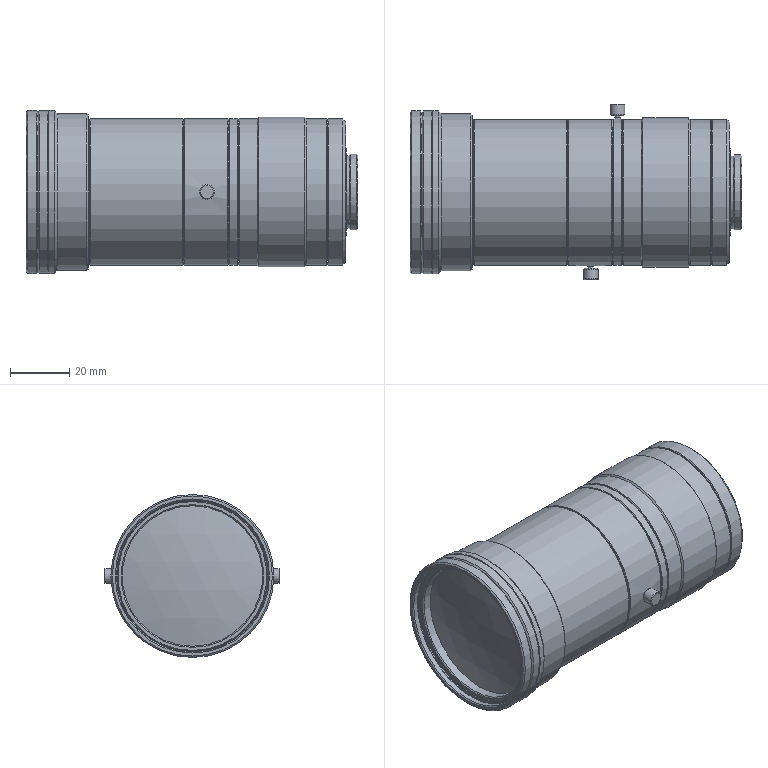Part | STEP file | VS-TEV0305-1-1-1 | 1 solid | 115 faces | box 111.97 x 59.35 x 55 mm | volume 201567 mm3 | cone 48 | cylinder 34 | plane 31 | sphere 2 | commonest cylinder face diameters 49.5 x6 55 x3 1.6 x2 2 x2 5 x2 20 x2